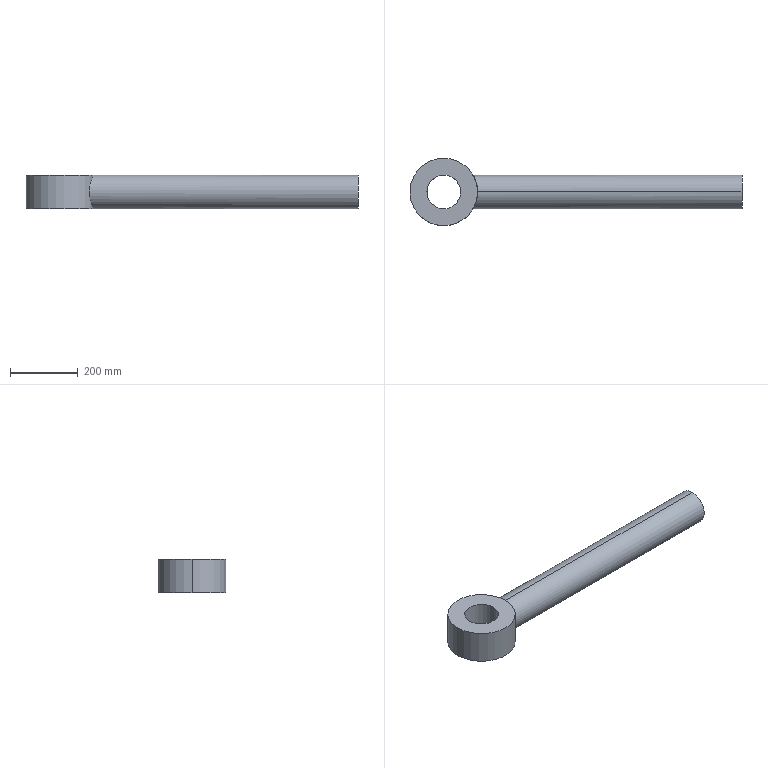Part | SolidWorks | features Extrusion 1, ICE 1 | 1 solid | 9 faces | box 982.338 x 200 x 100 mm | volume 8525978 mm3 | cylinder 6 | plane 3 | commonest cylinder face diameters 100 x4 200 x2
STEP:
#1=CARTESIAN_POINT('',(-132.338,0.,50.));
#2=VERTEX_POINT('',#1);
#3=CARTESIAN_POINT('',(-32.338,0.,50.));
#4=VERTEX_POINT('',#3);
#5=CARTESIAN_POINT('',(-82.338,0.,50.));
#6=DIRECTION('',(0.,0.,1.));
#7=DIRECTION('',(1.,0.,0.));
#8=AXIS2_PLACEMENT_3D('',#5,#6,#7);
#9=CIRCLE('',#8,50.);
#10=EDGE_CURVE('',#2,#4,#9,.T.);
#11=ORIENTED_EDGE('',*,*,#10,.T.);
#12=CARTESIAN_POINT('',(-32.338,0.,-50.));
#13=VERTEX_POINT('',#12);
#14=CARTESIAN_POINT('',(-32.338,0.,50.));
#15=DIRECTION('',(0.,0.,-1.));
#16=VECTOR('',#15,1000.);
#17=LINE('',#14,#16);
#18=EDGE_CURVE('',#4,#13,#17,.T.);
#19=ORIENTED_EDGE('',*,*,#18,.T.);
#20=CARTESIAN_POINT('',(-132.338,0.,-50.));
#21=VERTEX_POINT('',#20);
#22=CARTESIAN_POINT('',(-82.338,0.,-50.));
#23=DIRECTION('',(0.,0.,1.));
#24=DIRECTION('',(1.,0.,0.));
#25=AXIS2_PLACEMENT_3D('',#22,#23,#24);
#26=CIRCLE('',#25,50.);
#27=EDGE_CURVE('',#21,#13,#26,.T.);
#28=ORIENTED_EDGE('',*,*,#27,.F.);
#29=CARTESIAN_POINT('',(-132.338,0.,50.));
#30=DIRECTION('',(0.,0.,-1.));
#31=VECTOR('',#30,1000.);
#32=LINE('',#29,#31);
#33=EDGE_CURVE('',#2,#21,#32,.T.);
#34=ORIENTED_EDGE('',*,*,#33,.F.);
#35=EDGE_LOOP('',(#11,#19,#28,#34));
#36=FACE_OUTER_BOUND('',#35,.T.);
#37=CARTESIAN_POINT('',(-82.338,0.,50.));
#38=DIRECTION('',(0.,0.,-1.));
#39=DIRECTION('',(-1.,0.,0.));
#40=AXIS2_PLACEMENT_3D('',#37,#38,#39);
#41=CYLINDRICAL_SURFACE('',#40,50.);
#42=ADVANCED_FACE('',(#36),#41,.F.);
#43=CARTESIAN_POINT('',(-182.338,0.,50.));
#44=VERTEX_POINT('',#43);
#45=CARTESIAN_POINT('',(17.662,0.,50.));
#46=VERTEX_POINT('',#45);
#47=CARTESIAN_POINT('',(-82.338,0.,50.));
#48=DIRECTION('',(0.,0.,1.));
#49=DIRECTION('',(1.,0.,0.));
#50=AXIS2_PLACEMENT_3D('',#47,#48,#49);
#51=CIRCLE('',#50,100.);
#52=EDGE_CURVE('',#44,#46,#51,.T.);
#53=ORIENTED_EDGE('',*,*,#52,.F.);
#54=CARTESIAN_POINT('',(-182.338,0.,-50.));
#55=VERTEX_POINT('',#54);
#56=CARTESIAN_POINT('',(-182.338,0.,50.));
#57=DIRECTION('',(0.,0.,-1.));
#58=VECTOR('',#57,1000.);
#59=LINE('',#56,#58);
#60=EDGE_CURVE('',#44,#55,#59,.T.);
#61=ORIENTED_EDGE('',*,*,#60,.T.);
#62=CARTESIAN_POINT('',(17.662,0.,-50.));
#63=VERTEX_POINT('',#62);
#64=CARTESIAN_POINT('',(-82.338,0.,-50.));
#65=DIRECTION('',(0.,0.,1.));
#66=DIRECTION('',(1.,0.,0.));
#67=AXIS2_PLACEMENT_3D('',#64,#65,#66);
#68=CIRCLE('',#67,100.);
#69=EDGE_CURVE('',#55,#63,#68,.T.);
#70=ORIENTED_EDGE('',*,*,#69,.T.);
#71=CARTESIAN_POINT('',(17.662,0.,-50.));
#72=CARTESIAN_POINT('',(17.662,-1.657,-50.));
#73=CARTESIAN_POINT('',(17.621,-3.321,-49.918));
#74=CARTESIAN_POINT('',(17.454,-6.661,-49.583));
#75=CARTESIAN_POINT('',(17.33,-8.307,-49.333));
#76=CARTESIAN_POINT('',(16.845,-13.167,-48.348));
#77=CARTESIAN_POINT('',(16.372,-16.308,-47.381));
#78=CARTESIAN_POINT('',(15.621,-20.115,-45.783));
#79=CARTESIAN_POINT('',(15.464,-20.866,-45.445));
#80=CARTESIAN_POINT('',(15.137,-22.343,-44.738));
#81=CARTESIAN_POINT('',(14.968,-23.069,-44.367));
#82=CARTESIAN_POINT('',(14.443,-25.214,-43.208));
#83=CARTESIAN_POINT('',(14.07,-26.598,-42.37));
#84=CARTESIAN_POINT('',(13.291,-29.276,-40.565));
#85=CARTESIAN_POINT('',(12.884,-30.57,-39.599));
#86=CARTESIAN_POINT('',(12.254,-32.446,-38.051));
#87=CARTESIAN_POINT('',(12.041,-33.06,-37.519));
#88=CARTESIAN_POINT('',(11.614,-34.255,-36.431));
#89=CARTESIAN_POINT('',(11.4,-34.837,-35.875));
#90=CARTESIAN_POINT('',(10.326,-37.674,-33.031));
#91=CARTESIAN_POINT('',(9.463,-39.706,-30.559));
#92=CARTESIAN_POINT('',(8.436,-41.957,-27.208));
#93=CARTESIAN_POINT('',(8.233,-42.392,-26.525));
#94=CARTESIAN_POINT('',(7.835,-43.233,-25.131));
#95=CARTESIAN_POINT('',(7.64,-43.638,-24.422));
#96=CARTESIAN_POINT('',(7.073,-44.794,-22.275));
#97=CARTESIAN_POINT('',(6.718,-45.492,-20.812));
#98=CARTESIAN_POINT('',(5.742,-47.37,-16.328));
#99=CARTESIAN_POINT('',(5.207,-48.338,-13.211));
#100=CARTESIAN_POINT('',(4.741,-49.166,-9.135));
#101=CARTESIAN_POINT('',(4.659,-49.312,-8.308));
#102=CARTESIAN_POINT('',(4.517,-49.562,-6.66));
#103=CARTESIAN_POINT('',(4.457,-49.665,-5.835));
#104=CARTESIAN_POINT('',(4.314,-49.915,-3.359));
#105=CARTESIAN_POINT('',(4.266,-49.998,-1.708));
#106=CARTESIAN_POINT('',(4.264,-50.002,1.599));
#107=CARTESIAN_POINT('',(4.31,-49.922,3.254));
#108=CARTESIAN_POINT('',(4.451,-49.676,5.739));
#109=CARTESIAN_POINT('',(4.51,-49.574,6.568));
#110=CARTESIAN_POINT('',(4.651,-49.326,8.226));
#111=CARTESIAN_POINT('',(4.732,-49.182,9.047));
#112=CARTESIAN_POINT('',(5.192,-48.363,13.114));
#113=CARTESIAN_POINT('',(5.726,-47.4,16.248));
#114=CARTESIAN_POINT('',(6.547,-45.821,20.027));
#115=CARTESIAN_POINT('',(6.719,-45.486,20.778));
#116=CARTESIAN_POINT('',(7.077,-44.78,22.258));
#117=CARTESIAN_POINT('',(7.261,-44.41,22.986));
#118=CARTESIAN_POINT('',(7.828,-43.255,25.133));
#119=CARTESIAN_POINT('',(8.224,-42.42,26.516));
#120=CARTESIAN_POINT('',(9.043,-40.626,29.19));
#121=CARTESIAN_POINT('',(9.465,-39.667,30.482));
#122=CARTESIAN_POINT('',(10.108,-38.132,32.351));
#123=CARTESIAN_POINT('',(10.324,-37.604,32.963));
#124=CARTESIAN_POINT('',(10.759,-36.516,34.165));
#125=CARTESIAN_POINT('',(10.976,-35.958,34.752));
#126=CARTESIAN_POINT('',(12.054,-33.108,37.606));
#127=CARTESIAN_POINT('',(12.895,-30.635,39.647));
#128=CARTESIAN_POINT('',(14.063,-26.622,42.354));
#129=CARTESIAN_POINT('',(14.438,-25.234,43.197));
#130=CARTESIAN_POINT('',(14.968,-23.07,44.367));
#131=CARTESIAN_POINT('',(15.139,-22.337,44.741));
#132=CARTESIAN_POINT('',(15.465,-20.86,45.448));
#133=CARTESIAN_POINT('',(15.621,-20.114,45.783));
#134=CARTESIAN_POINT('',(16.364,-16.351,47.364));
#135=CARTESIAN_POINT('',(16.837,-13.227,48.332));
#136=CARTESIAN_POINT('',(17.244,-9.17,49.159));
#137=CARTESIAN_POINT('',(17.316,-8.351,49.305));
#138=CARTESIAN_POINT('',(17.441,-6.697,49.557));
#139=CARTESIAN_POINT('',(17.494,-5.862,49.662));
#140=CARTESIAN_POINT('',(17.578,-4.193,49.831));
#141=CARTESIAN_POINT('',(17.609,-3.357,49.894));
#142=CARTESIAN_POINT('',(17.652,-1.681,49.979));
#143=CARTESIAN_POINT('',(17.662,-0.8398,50.));
#144=CARTESIAN_POINT('',(17.662,0.,50.));
#145=B_SPLINE_CURVE_WITH_KNOTS('',3,(#71,#72,#73,#74,#75,#76,#77,#78,#79,#80,#81,#82,#83,#84,#85,#86,#87,#88,#89,#90,#91,#92,#93,#94,#95,#96,#97,#98,#99,#100,#101,#102,#103,#104,#105,#106,#107,#108,#109,#110,#111,#112,#113,#114,#115,#116,#117,#118,#119,#120,#121,#122,#123,#124,#125,#126,#127,#128,#129,#130,#131,#132,#133,#134,#135,#136,#137,#138,#139,#140,#141,#142,#143,#144),.UNSPECIFIED.,.F.,.F.,(4,2,2,2,2,2,2,2,2,2,2,2,2,2,2,2,2,2,2,2,2,2,2,2,2,2,2,2,2,2,2,2,2,2,2,2,4),(0.159,0.164,0.169,0.1789,0.1814,0.1839,0.1888,0.1938,0.1963,0.1987,0.2087,0.2111,0.2136,0.2186,0.2285,0.231,0.2335,0.2384,0.2434,0.2459,0.2484,0.2583,0.2608,0.2632,0.2682,0.2732,0.2756,0.2781,0.2881,0.293,0.2955,0.298,0.3079,0.3104,0.3129,0.3153,0.3178),.UNSPECIFIED.);
#146=EDGE_CURVE('',#63,#46,#145,.T.);
#147=ORIENTED_EDGE('',*,*,#146,.T.);
#148=EDGE_LOOP('',(#53,#61,#70,#147));
#149=FACE_OUTER_BOUND('',#148,.T.);
#150=CARTESIAN_POINT('',(-82.338,0.,50.));
#151=DIRECTION('',(0.,0.,-1.));
#152=DIRECTION('',(-1.,0.,0.));
#153=AXIS2_PLACEMENT_3D('',#150,#151,#152);
#154=CYLINDRICAL_SURFACE('',#153,100.);
#155=ADVANCED_FACE('',(#149),#154,.T.);
#156=CARTESIAN_POINT('',(800.,0.,-50.));
#157=VERTEX_POINT('',#156);
#158=CARTESIAN_POINT('',(800.,0.,50.));
#159=VERTEX_POINT('',#158);
#160=CARTESIAN_POINT('',(800.,0.,0.));
#161=DIRECTION('',(1.,0.,0.));
#162=DIRECTION('',(0.,0.,-1.));
#163=AXIS2_PLACEMENT_3D('',#160,#161,#162);
#164=CIRCLE('',#163,50.);
#165=EDGE_CURVE('',#157,#159,#164,.T.);
#166=ORIENTED_EDGE('',*,*,#165,.F.);
#167=CARTESIAN_POINT('',(800.,0.,-50.));
#168=DIRECTION('',(-1.,0.,0.));
#169=VECTOR('',#168,1000.);
#170=LINE('',#167,#169);
#171=EDGE_CURVE('',#157,#63,#170,.T.);
#172=ORIENTED_EDGE('',*,*,#171,.T.);
#173=CARTESIAN_POINT('',(17.662,0.,50.));
#174=CARTESIAN_POINT('',(17.662,3.365,50.));
#175=CARTESIAN_POINT('',(17.493,6.663,49.664));
#176=CARTESIAN_POINT('',(17.01,11.517,48.683));
#177=CARTESIAN_POINT('',(16.811,13.12,48.277));
#178=CARTESIAN_POINT('',(16.457,15.5,47.544));
#179=CARTESIAN_POINT('',(16.33,16.289,47.28));
#180=CARTESIAN_POINT('',(16.061,17.841,46.716));
#181=CARTESIAN_POINT('',(15.919,18.606,46.416));
#182=CARTESIAN_POINT('',(15.174,22.38,44.831));
#183=CARTESIAN_POINT('',(14.467,25.234,43.288));
#184=CARTESIAN_POINT('',(13.486,28.606,41.017));
#185=CARTESIAN_POINT('',(13.284,29.272,40.544));
#186=CARTESIAN_POINT('',(12.876,30.574,39.571));
#187=CARTESIAN_POINT('',(12.669,31.21,39.071));
#188=CARTESIAN_POINT('',(12.043,33.076,37.531));
#189=CARTESIAN_POINT('',(11.617,34.263,36.45));
#190=CARTESIAN_POINT('',(10.76,36.528,34.18));
#191=CARTESIAN_POINT('',(10.329,37.605,32.992));
#192=CARTESIAN_POINT('',(9.686,39.139,31.125));
#193=CARTESIAN_POINT('',(9.473,39.637,30.489));
#194=CARTESIAN_POINT('',(9.049,40.605,29.188));
#195=CARTESIAN_POINT('',(8.839,41.074,28.523));
#196=CARTESIAN_POINT('',(7.809,43.329,25.16));
#197=CARTESIAN_POINT('',(7.048,44.858,22.323));
#198=CARTESIAN_POINT('',(6.069,46.741,17.831));
#199=CARTESIAN_POINT('',(5.771,47.299,16.294));
#200=CARTESIAN_POINT('',(5.374,48.029,13.924));
#201=CARTESIAN_POINT('',(5.249,48.255,13.121));
#202=CARTESIAN_POINT('',(5.023,48.664,11.513));
#203=CARTESIAN_POINT('',(4.92,48.847,10.706));
#204=CARTESIAN_POINT('',(4.461,49.665,6.658));
#205=CARTESIAN_POINT('',(4.267,49.997,3.376));
#206=CARTESIAN_POINT('',(4.264,50.001,-0.7836));
#207=CARTESIAN_POINT('',(4.276,49.981,-1.618));
#208=CARTESIAN_POINT('',(4.323,49.898,-3.294));
#209=CARTESIAN_POINT('',(4.359,49.836,-4.134));
#210=CARTESIAN_POINT('',(4.502,49.587,-6.628));
#211=CARTESIAN_POINT('',(4.644,49.339,-8.268));
#212=CARTESIAN_POINT('',(5.011,48.687,-11.504));
#213=CARTESIAN_POINT('',(5.236,48.282,-13.099));
#214=CARTESIAN_POINT('',(5.631,47.557,-15.461));
#215=CARTESIAN_POINT('',(5.772,47.295,-16.243));
#216=CARTESIAN_POINT('',(6.071,46.733,-17.796));
#217=CARTESIAN_POINT('',(6.229,46.432,-18.566));
#218=CARTESIAN_POINT('',(7.053,44.847,-22.349));
#219=CARTESIAN_POINT('',(7.82,43.308,-25.197));
#220=CARTESIAN_POINT('',(8.848,41.054,-28.552));
#221=CARTESIAN_POINT('',(9.057,40.586,-29.213));
#222=CARTESIAN_POINT('',(9.481,39.617,-30.515));
#223=CARTESIAN_POINT('',(9.696,39.115,-31.155));
#224=CARTESIAN_POINT('',(10.342,37.574,-33.028));
#225=CARTESIAN_POINT('',(10.774,36.493,-34.218));
#226=CARTESIAN_POINT('',(12.06,33.09,-37.621));
#227=CARTESIAN_POINT('',(12.903,30.612,-39.668));
#228=CARTESIAN_POINT('',(13.887,27.227,-41.945));
#229=CARTESIAN_POINT('',(14.08,26.537,-42.385));
#230=CARTESIAN_POINT('',(14.453,25.142,-43.226));
#231=CARTESIAN_POINT('',(14.633,24.436,-43.629));
#232=CARTESIAN_POINT('',(15.157,22.292,-44.785));
#233=CARTESIAN_POINT('',(15.481,20.827,-45.485));
#234=CARTESIAN_POINT('',(16.073,17.826,-46.743));
#235=CARTESIAN_POINT('',(16.34,16.289,-47.301));
#236=CARTESIAN_POINT('',(16.691,13.927,-48.028));
#237=CARTESIAN_POINT('',(16.8,13.13,-48.252));
#238=CARTESIAN_POINT('',(17.,11.517,-48.663));
#239=CARTESIAN_POINT('',(17.092,10.699,-48.849));
#240=CARTESIAN_POINT('',(17.497,6.614,-49.673));
#241=CARTESIAN_POINT('',(17.662,3.32,-50.));
#242=CARTESIAN_POINT('',(17.662,0.,-50.));
#243=B_SPLINE_CURVE_WITH_KNOTS('',3,(#173,#174,#175,#176,#177,#178,#179,#180,#181,#182,#183,#184,#185,#186,#187,#188,#189,#190,#191,#192,#193,#194,#195,#196,#197,#198,#199,#200,#201,#202,#203,#204,#205,#206,#207,#208,#209,#210,#211,#212,#213,#214,#215,#216,#217,#218,#219,#220,#221,#222,#223,#224,#225,#226,#227,#228,#229,#230,#231,#232,#233,#234,#235,#236,#237,#238,#239,#240,#241,#242),.UNSPECIFIED.,.F.,.F.,(4,2,2,2,2,2,2,2,2,2,2,2,2,2,2,2,2,2,2,2,2,2,2,2,2,2,2,2,2,2,2,2,2,2,4),(0.,0.009941,0.01491,0.0174,0.01988,0.02982,0.03231,0.03479,0.03976,0.04473,0.04722,0.0497,0.05964,0.06461,0.0671,0.06958,0.07952,0.08201,0.08449,0.08947,0.09444,0.09692,0.09941,0.1093,0.1118,0.1143,0.1193,0.1292,0.1317,0.1342,0.1392,0.1441,0.1466,0.1491,0.159),.UNSPECIFIED.);
#244=EDGE_CURVE('',#46,#63,#243,.T.);
#245=ORIENTED_EDGE('',*,*,#244,.F.);
#246=CARTESIAN_POINT('',(800.,0.,50.));
#247=DIRECTION('',(-1.,0.,0.));
#248=VECTOR('',#247,1000.);
#249=LINE('',#246,#248);
#250=EDGE_CURVE('',#159,#46,#249,.T.);
#251=ORIENTED_EDGE('',*,*,#250,.F.);
#252=EDGE_LOOP('',(#166,#172,#245,#251));
#253=FACE_OUTER_BOUND('',#252,.T.);
#254=CARTESIAN_POINT('',(800.,0.,0.));
#255=DIRECTION('',(-1.,0.,0.));
#256=DIRECTION('',(0.,0.,1.));
#257=AXIS2_PLACEMENT_3D('',#254,#255,#256);
#258=CYLINDRICAL_SURFACE('',#257,50.);
#259=ADVANCED_FACE('',(#253),#258,.T.);
#260=ORIENTED_EDGE('',*,*,#171,.F.);
#261=CARTESIAN_POINT('',(800.,0.,0.));
#262=DIRECTION('',(1.,0.,0.));
#263=DIRECTION('',(0.,0.,-1.));
#264=AXIS2_PLACEMENT_3D('',#261,#262,#263);
#265=CIRCLE('',#264,50.);
#266=EDGE_CURVE('',#159,#157,#265,.T.);
#267=ORIENTED_EDGE('',*,*,#266,.F.);
#268=ORIENTED_EDGE('',*,*,#250,.T.);
#269=ORIENTED_EDGE('',*,*,#146,.F.);
#270=EDGE_LOOP('',(#260,#267,#268,#269));
#271=FACE_OUTER_BOUND('',#270,.T.);
#272=CARTESIAN_POINT('',(800.,0.,0.));
#273=DIRECTION('',(-1.,0.,0.));
#274=DIRECTION('',(0.,0.,1.));
#275=AXIS2_PLACEMENT_3D('',#272,#273,#274);
#276=CYLINDRICAL_SURFACE('',#275,50.);
#277=ADVANCED_FACE('',(#271),#276,.T.);
#278=ORIENTED_EDGE('',*,*,#266,.T.);
#279=ORIENTED_EDGE('',*,*,#165,.T.);
#280=EDGE_LOOP('',(#278,#279));
#281=FACE_OUTER_BOUND('',#280,.T.);
#282=CARTESIAN_POINT('',(800.,0.,0.));
#283=DIRECTION('',(1.,0.,0.));
#284=DIRECTION('',(0.,0.,-1.));
#285=AXIS2_PLACEMENT_3D('',#282,#283,#284);
#286=PLANE('',#285);
#287=ADVANCED_FACE('',(#281),#286,.T.);
#288=ORIENTED_EDGE('',*,*,#60,.F.);
#289=CARTESIAN_POINT('',(-82.338,0.,50.));
#290=DIRECTION('',(0.,0.,1.));
#291=DIRECTION('',(1.,0.,0.));
#292=AXIS2_PLACEMENT_3D('',#289,#290,#291);
#293=CIRCLE('',#292,100.);
#294=EDGE_CURVE('',#46,#44,#293,.T.);
#295=ORIENTED_EDGE('',*,*,#294,.F.);
#296=ORIENTED_EDGE('',*,*,#244,.T.);
#297=CARTESIAN_POINT('',(-82.338,0.,-50.));
#298=DIRECTION('',(0.,0.,1.));
#299=DIRECTION('',(1.,0.,0.));
#300=AXIS2_PLACEMENT_3D('',#297,#298,#299);
#301=CIRCLE('',#300,100.);
#302=EDGE_CURVE('',#63,#55,#301,.T.);
#303=ORIENTED_EDGE('',*,*,#302,.T.);
#304=EDGE_LOOP('',(#288,#295,#296,#303));
#305=FACE_OUTER_BOUND('',#304,.T.);
#306=CARTESIAN_POINT('',(-82.338,0.,50.));
#307=DIRECTION('',(0.,0.,-1.));
#308=DIRECTION('',(-1.,0.,0.));
#309=AXIS2_PLACEMENT_3D('',#306,#307,#308);
#310=CYLINDRICAL_SURFACE('',#309,100.);
#311=ADVANCED_FACE('',(#305),#310,.T.);
#312=ORIENTED_EDGE('',*,*,#294,.T.);
#313=ORIENTED_EDGE('',*,*,#52,.T.);
#314=EDGE_LOOP('',(#312,#313));
#315=FACE_OUTER_BOUND('',#314,.T.);
#316=ORIENTED_EDGE('',*,*,#10,.F.);
#317=CARTESIAN_POINT('',(-82.338,0.,50.));
#318=DIRECTION('',(0.,0.,1.));
#319=DIRECTION('',(1.,0.,0.));
#320=AXIS2_PLACEMENT_3D('',#317,#318,#319);
#321=CIRCLE('',#320,50.);
#322=EDGE_CURVE('',#4,#2,#321,.T.);
#323=ORIENTED_EDGE('',*,*,#322,.F.);
#324=EDGE_LOOP('',(#316,#323));
#325=FACE_BOUND('',#324,.T.);
#326=CARTESIAN_POINT('',(-82.338,0.,50.));
#327=DIRECTION('',(0.,0.,1.));
#328=DIRECTION('',(1.,0.,0.));
#329=AXIS2_PLACEMENT_3D('',#326,#327,#328);
#330=PLANE('',#329);
#331=ADVANCED_FACE('',(#315,#325),#330,.T.);
#332=ORIENTED_EDGE('',*,*,#302,.F.);
#333=ORIENTED_EDGE('',*,*,#69,.F.);
#334=EDGE_LOOP('',(#332,#333));
#335=FACE_OUTER_BOUND('',#334,.T.);
#336=ORIENTED_EDGE('',*,*,#27,.T.);
#337=CARTESIAN_POINT('',(-82.338,0.,-50.));
#338=DIRECTION('',(0.,0.,1.));
#339=DIRECTION('',(1.,0.,0.));
#340=AXIS2_PLACEMENT_3D('',#337,#338,#339);
#341=CIRCLE('',#340,50.);
#342=EDGE_CURVE('',#13,#21,#341,.T.);
#343=ORIENTED_EDGE('',*,*,#342,.T.);
#344=EDGE_LOOP('',(#336,#343));
#345=FACE_BOUND('',#344,.T.);
#346=CARTESIAN_POINT('',(-82.338,0.,-50.));
#347=DIRECTION('',(0.,0.,1.));
#348=DIRECTION('',(1.,0.,0.));
#349=AXIS2_PLACEMENT_3D('',#346,#347,#348);
#350=PLANE('',#349);
#351=ADVANCED_FACE('',(#335,#345),#350,.F.);
#352=ORIENTED_EDGE('',*,*,#18,.F.);
#353=ORIENTED_EDGE('',*,*,#322,.T.);
#354=ORIENTED_EDGE('',*,*,#33,.T.);
#355=ORIENTED_EDGE('',*,*,#342,.F.);
#356=EDGE_LOOP('',(#352,#353,#354,#355));
#357=FACE_OUTER_BOUND('',#356,.T.);
#358=CARTESIAN_POINT('',(-82.338,0.,50.));
#359=DIRECTION('',(0.,0.,-1.));
#360=DIRECTION('',(-1.,0.,0.));
#361=AXIS2_PLACEMENT_3D('',#358,#359,#360);
#362=CYLINDRICAL_SURFACE('',#361,50.);
#363=ADVANCED_FACE('',(#357),#362,.F.);
#364=CLOSED_SHELL('',(#42,#155,#259,#277,#287,#311,#331,#351,#363));
#365=MANIFOLD_SOLID_BREP('',#364);
#366=CARTESIAN_POINT('',(0.,0.,0.));
#367=DIRECTION('',(0.,0.,1.));
#368=DIRECTION('',(1.,0.,0.));
#369=AXIS2_PLACEMENT_3D('',#366,#367,#368);
#370=(LENGTH_UNIT()NAMED_UNIT(*)SI_UNIT(.MILLI.,.METRE.));
#371=UNCERTAINTY_MEASURE_WITH_UNIT(LENGTH_MEASURE(0.00001),#370,'','');
#372=(NAMED_UNIT(*)PLANE_ANGLE_UNIT()SI_UNIT($,.RADIAN.));
#373=(NAMED_UNIT(*)SI_UNIT($,.STERADIAN.)SOLID_ANGLE_UNIT());
#374=(GEOMETRIC_REPRESENTATION_CONTEXT(3)GLOBAL_UNCERTAINTY_ASSIGNED_CONTEXT((#371))GLOBAL_UNIT_ASSIGNED_CONTEXT((#370,#372,#373))REPRESENTATION_CONTEXT('',''));
#375=ADVANCED_BREP_SHAPE_REPRESENTATION('',(#365,#369),#374);